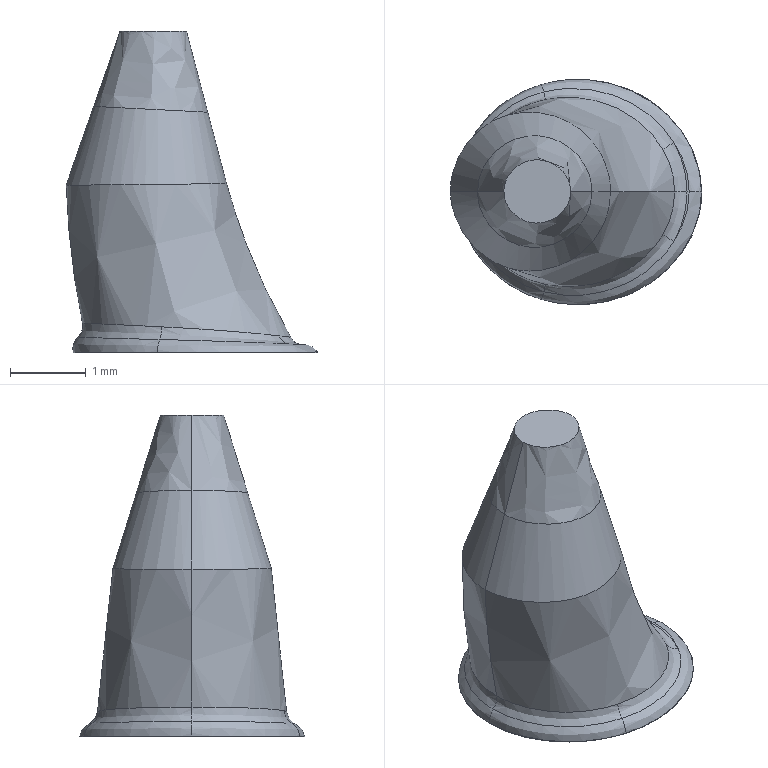Part | STEP file | solid 202 | 1 solid | 23 faces | box 3.318 x 2.972 x 4.241 mm | volume 13.916 mm3 | spline 20 | plane 3